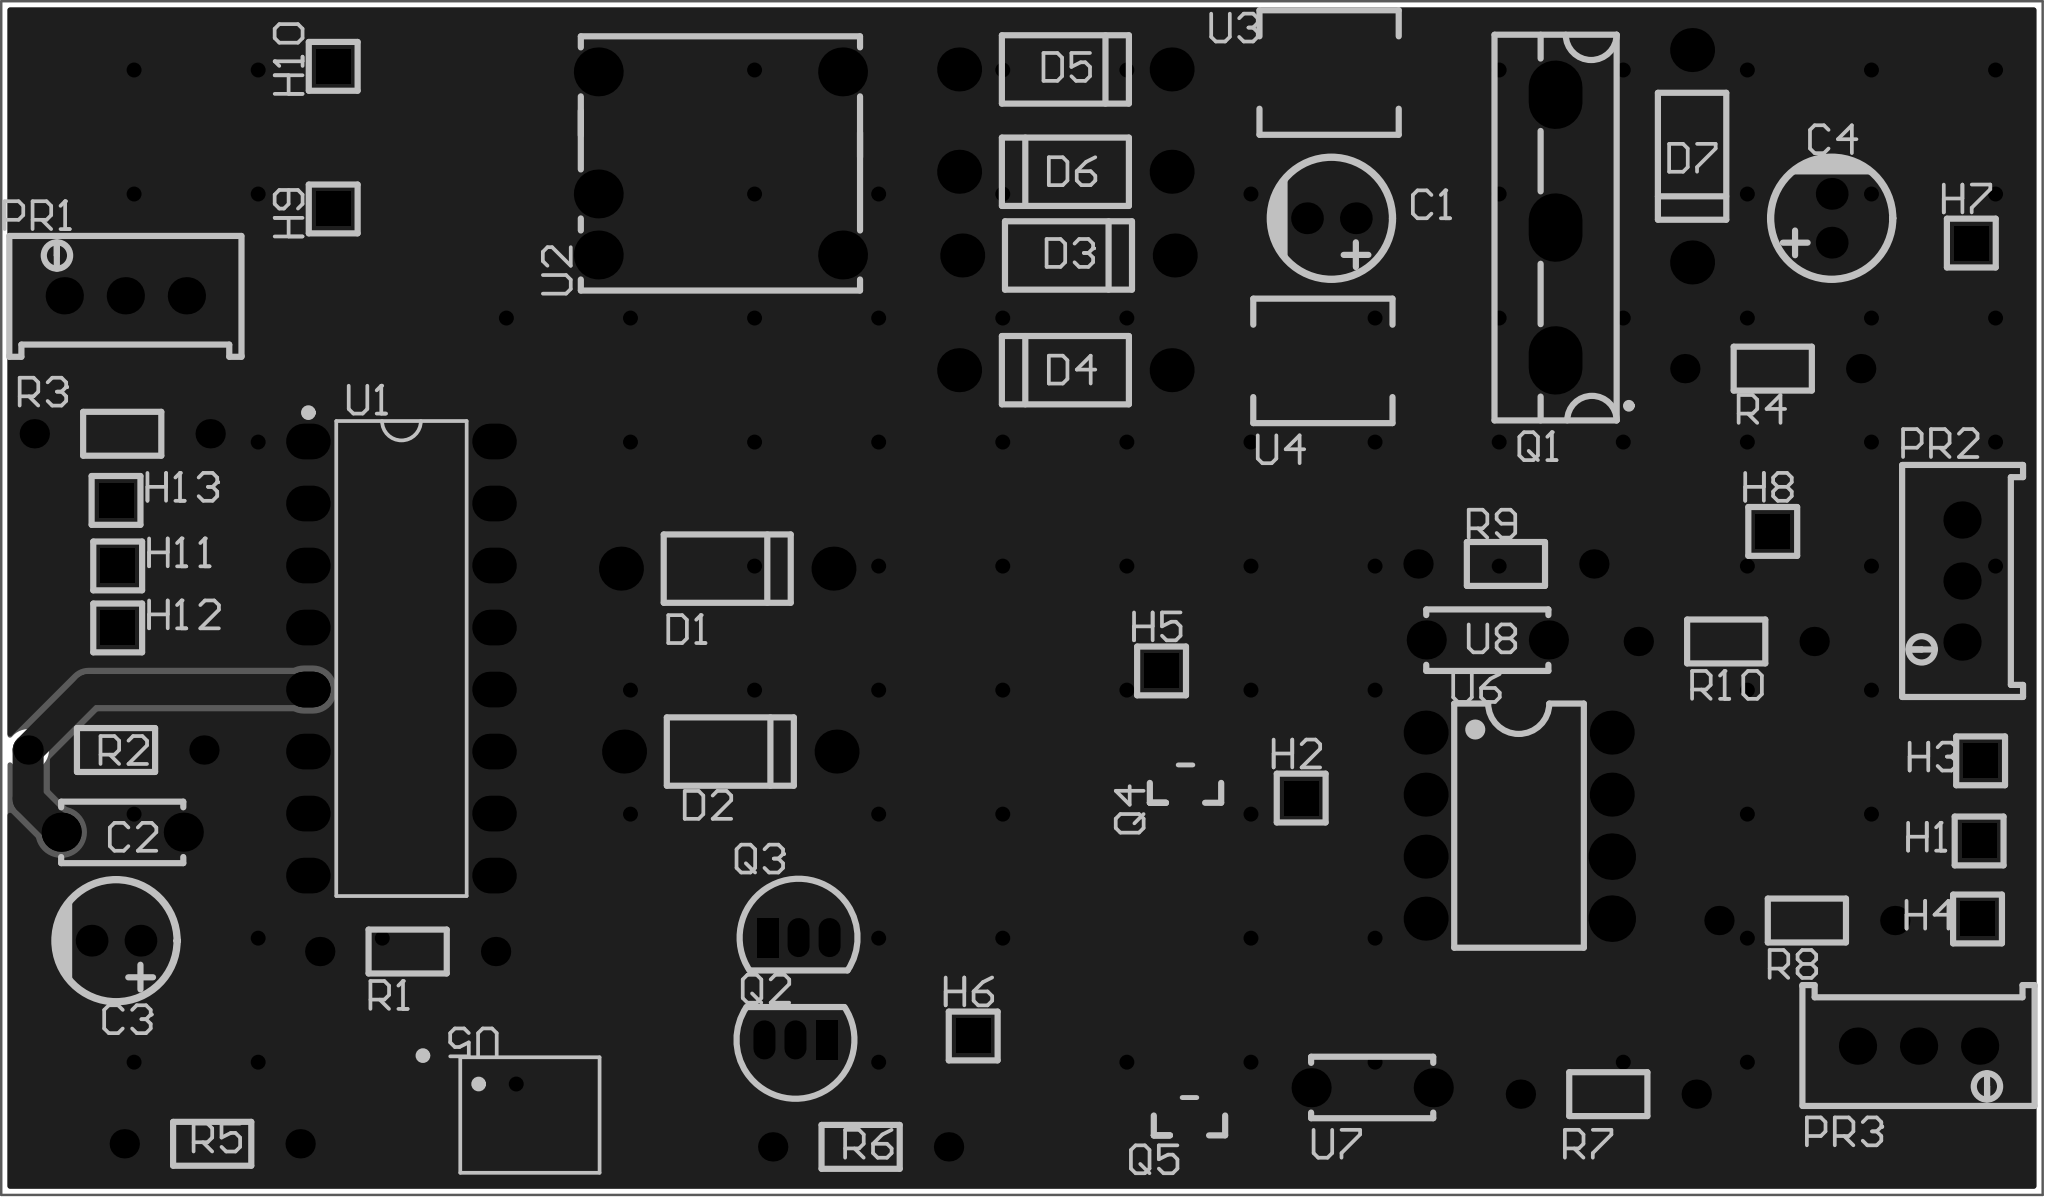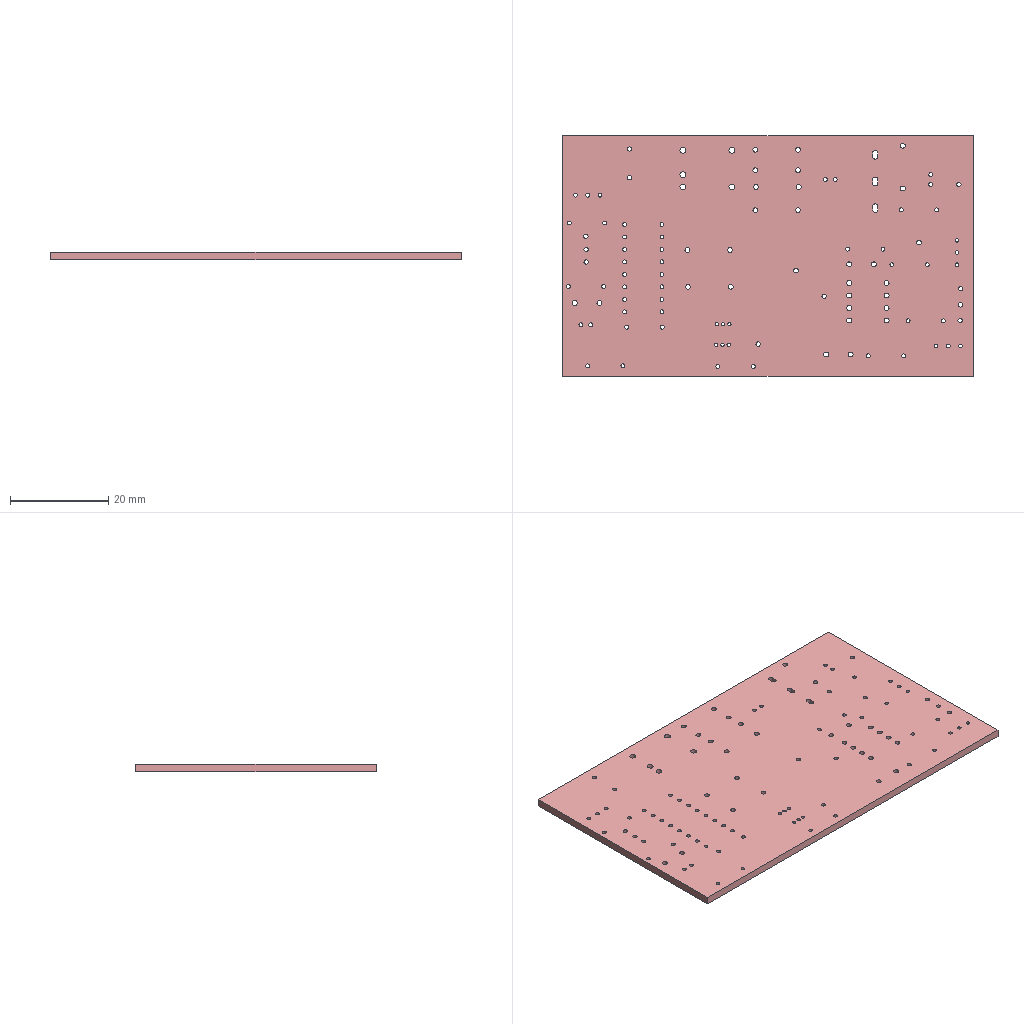Circuit board layout | Altium Designer | box 83.6 x 48.9 x 1.6 mm
Layer stack:
# Altium Designer layer stack of  (unit mm; dielectric type: 0 none, 1 core, 2 prepreg, 3 surface material)
index,name,kind,layer,copper_thickness_mm,dielectric_type,dielectric_thickness_mm,dielectric_material,dielectric_constant
0,Top Paste Mask Layer,other,,,,,,
1,Top Silkscreen Layer,other,,,,,,
2,Top Solder Mask Layer,dielectric,,,3,0.01,,3.3
3,Top Layer,copper,Top Layer,0.035,,,,
4,Dielectric1,dielectric,,,3,1.51,FR4,4.5
5,Bottom Layer,copper,Bottom Layer,0.035,,,,
6,Bottom Solder Mask Layer,dielectric,,,3,0.01,,3.3
7,Bottom Silkscreen Layer,other,,,,,,
8,Bottom Paste Mask Layer,other,,,,,,
# drill layer pairs: low layer,high layer
drill_pair,Top Layer,Bottom Layer
Part placement:
Designator,Comment,Layer,Footprint,Center-X(mm),Center-Y(mm),Rotation
C1,10uF,TopLayer,CAP-TH_BD5.0-P2.00-D0.8-FD-10UF50VC110GL,136.112,123.825,180
C2,100nF,TopLayer,CAP-TH_L5.0-W2.5-P5.00-D1.0,86.614,98.679,0
C3,10uF,TopLayer,CAP-TH_BD5.0-P2.00-D0.8-FD-10UF50VC110GL,86.36,94.234,180
C4,10uF,TopLayer,CAP-TH_BD5.0-P2.00-D0.8-FD-10UF50VC110GL,156.591,123.825,90
D1,,TopLayer,DO_1N4007,111.379,109.474,180
D2,,TopLayer,DO_1N4007,111.506,101.981,180
D3,,TopLayer,DO_1N4007,125.349,122.301,180
D4,,TopLayer,DO_1N4007,125.222,117.602,0
D5,,TopLayer,DO_1N4007,125.222,129.921,180
D6,,TopLayer,DO_1N4007,125.222,125.73,0
D7,,TopLayer,DO_1N4007,150.876,126.365,90
H1,,TopLayer,HDR-TH_1P-V-M_XKB_X4611WV-01I-C28D40,162.625,98.319,0
H2,,TopLayer,HDR-TH_1P-V-M_XKB_X4611WV-01I-C28D40,134.874,100.076,0
H3,,TopLayer,HDR-TH_1P-V-M_XKB_X4611WV-01I-C28D40,162.687,101.6,0
H4,,TopLayer,HDR-TH_1P-V-M_XKB_X4611WV-01I-C28D40,162.56,95.123,0
H5,,TopLayer,HDR-TH_1P-V-M_XKB_X4611WV-01I-C28D40,129.159,105.283,0
H6,,TopLayer,HDR-TH_1P-V-M_XKB_X4611WV-01I-C28D40,121.448,90.331,0
H7,,TopLayer,HDR-TH_1P-V-M_XKB_X4611WV-01I-C28D40,162.306,122.809,0
H8,,TopLayer,HDR-TH_1P-V-M_XKB_X4611WV-01I-C28D40,154.178,110.998,0
H9,,TopLayer,HDR-TH_1P-V-M_XKB_X4611WV-01I-C28D40,95.25,124.206,90
H10,,TopLayer,HDR-TH_1P-V-M_XKB_X4611WV-01I-C28D40,95.25,130.048,90
H11,,TopLayer,HDR-TH_1P-V-M_XKB_X4611WV-01I-C28D40,86.428,109.584,0
H12,,TopLayer,HDR-TH_1P-V-M_XKB_X4611WV-01I-C28D40,86.428,107.044,0
H13,,TopLayer,HDR-TH_1P-V-M_XKB_X4611WV-01I-C28D40,86.36,112.268,0
PR1,10kΩ,TopLayer,R_3296,86.741,120.65,0
PR2,10kΩ,TopLayer,R_3296,161.925,108.966,90
PR3,10kΩ,TopLayer,R_3296,160.147,89.916,180
Q1,IGBT,TopLayer,TO-247-3_L15.9-W5.0-P5.44-L,145.288,123.444,90
Q2,,TopLayer,S8050_TO_92,114.173,90.17,180
Q3,,TopLayer,S8050_TO_92,114.3,94.361,0
Q4,,TopLayer,S8550P_SOT,130.14,100.534,90
Q5,,TopLayer,S8550P_SOT,130.302,86.91,90
R1,10kΩ,TopLayer,Res_1/8W,98.298,93.79,180
R2,10kΩ,TopLayer,Res_1/8W,86.36,102.044,0
R3,10kΩ,TopLayer,Res_1/8W,86.614,114.998,0
R4,10kΩ,TopLayer,Res_1/8W,154.178,117.666,180
R5,10kΩ,TopLayer,Res_1/8W,90.297,85.915,0
R6,10kΩ,TopLayer,Res_1/8W,116.84,85.789,180
R7,10kΩ,TopLayer,Res_1/8W,147.447,87.948,180
R8,10kΩ,TopLayer,Res_1/8W,155.575,95.06,180
R9,10kΩ,TopLayer,Res_1/8W,143.256,109.665,180
R10,10kΩ,TopLayer,Res_1/8W,152.273,106.49,180
U1,SG3525,TopLayer,DIP-16_L19.2-W6.6-P2.54-LS7.6-BL,98.044,105.791,270
U2,LT11-201G,TopLayer,XFMR-TH_LT13-201,111.101,126.071,90
U3,Power inductor (SMD), CKST0502-10uH/M, 10uH, ±20%, 3A, package 5.7mm*5.1mm*2.0mm, Cenke, RoHS,TopLayer,IND-SMD_L5.7-W5.1,136.017,129.794,0
U4,Power inductor (SMD), CKST0502-10uH/M, 10uH, ±20%, 3A, package 5.7mm*5.1mm*2.0mm, Cenke, RoHS,TopLayer,IND-SMD_L5.7-W5.1,135.763,117.983,0
U5,TLP521,TopLayer,SOP-4_L6.4-W4.6-P2.54-LS10.2-TL,103.303,87.093,0
U6,NE5532AP,TopLayer,PDIP-8_L9.6-W6.4-P2.54-LS7.6-BL,143.779,98.947,270
U7,100nF,TopLayer,CAP-TH_L5.0-W2.5-P5.00-D1.0,137.78,88.212,180
U8,100nF,TopLayer,CAP-TH_L5.0-W2.5-P5.00-D1.0,142.494,106.553,0
Pad and via stacks:
# Altium Designer via and pad stacks of  (unit mm). Each distinct definition once, with the count of objects using it.
# via: kind,start_layer,end_layer,hole_mm,diameter_mm,mode(0 simple;1 top-mid-bottom;2 full stack),diameter_per_layer,count,example_net
# pad: kind,layer,hole_mm,hole_type(0 round;1 square;2 slot),plating,top_size,top_shape(1 round;2 rect;3 octagon;9 rounded rect),mid_size,bottom_size,mode,footprint,size_per_layer,count,example
pad,Multi-Layer,0.8,0,plated,1.3x1.3,1,1.3x1.3,1.3x1.3,0,CAP-TH_BD5.0-P2.00-D0.8-FD-10UF50VC110GL,,6,C1.2
pad,Multi-Layer,1,0,plated,1.6x1.6,1,1.6x1.6,1.6x1.6,0,CAP-TH_L5.0-W2.5-P5.00-D1.0,,6,C2.1
pad,Multi-Layer,1,0,plated,1.8x1.8,1,1.8x1.8,1.8x1.8,0,DO_1N4007,,14,D1.1
pad,Multi-Layer,0.9,0,plated,1.4x1.4,2,1.4x1.4,1.4x1.4,0,HDR-TH_1P-V-M_XKB_X4611WV-01I-C28D40,,13,H1.1
pad,Multi-Layer,0.762,0,plated,1.524x1.524,1,1.524x1.524,1.524x1.524,0,R_3296,,9,PR1.2
pad,Multi-Layer,1,2,plated,2.8x2.2,1,2.8x2.2,2.8x2.2,0,TO-247-3_L15.9-W5.0-P5.44-L,,3,Q1.3
pad,Multi-Layer,0.701,0,plated,0.8992x1.6,2,0.8992x1.6,0.8992x1.6,0,S8050_TO_92,,2,Q2.1
pad,Multi-Layer,0.701,0,plated,0.8992x1.6,1,0.8992x1.6,0.8992x1.6,0,S8050_TO_92,,4,Q2.2
pad,Multi-Layer,0.8001,0,plated,1.199x1.199,1,1.199x1.199,1.199x1.199,0,Res_1/8W,,20,R1.1
pad,Multi-Layer,0.8,0,plated,1.46x1.825,1,1.46x1.825,1.46x1.825,0,DIP-16_L19.2-W6.6-P2.54-LS7.6-BL,,16,U1.1
pad,Multi-Layer,1.2,0,plated,2x2,1,2x2,2x2,0,XFMR-TH_LT13-201,,5,U2.1
pad,Multi-Layer,1,0,plated,1.8x1.8,1,1.8x1.8,1.8x1.8,0,PDIP-8_L9.6-W6.4-P2.54-LS7.6-BL,,6,U6.1
pad,Multi-Layer,1,0,plated,1.905x1.905,1,1.905x1.905,1.905x1.905,0,PDIP-8_L9.6-W6.4-P2.54-LS7.6-BL,,2,U6.5
pad,Top Layer,0,0,plated,0.701x1.25,2,0.701x1.25,0.701x1.25,0,S8550P_SOT,,6,Q4.3
pad,Top Layer,0,0,plated,2x2.5,2,2x2.5,2x2.5,0,IND-SMD_L5.7-W5.1,,4,U3.1
pad,Top Layer,0,0,plated,1.422x2.6,2,1.422x2.6,1.422x2.6,0,SOP-4_L6.4-W4.6-P2.54-LS10.2-TL,,4,U5.1
via,Top Layer,Bottom Layer,0.3048,0.61,0,,87,PWM
Copper pours:
name,layer,net,type(0 solid;1 hatched;2 none)
Top Layer-GND,Top Layer,GND,0
Bottom Layer-GND,Bottom Layer,GND,0
Design rules, without the lines most boards share:
# Altium Designer design rules of  (exported by Altium Designer, unit mm)
# columns: name | kind | enabled | priority | scope1 | scope2 | descriptor | typed fields (field=value)
creepage | 65 | enabled | 1 | All | All | Creepage Distance Constraint =(0mil) (All),(All) |